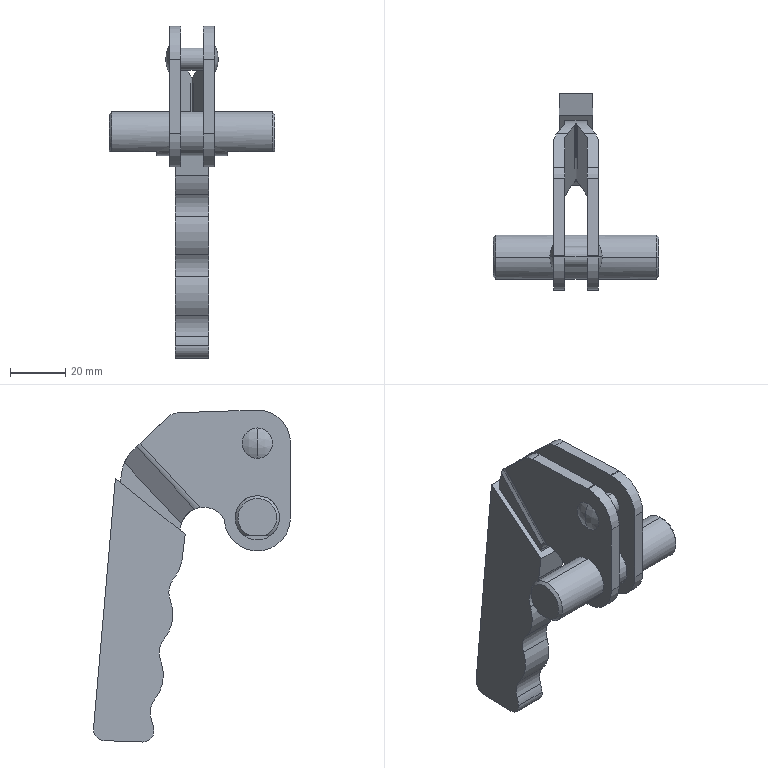Part | STEP file | _2-QC-408710.step | 1 solid | 72 faces | box 60 x 71.267 x 120.088 mm | volume 53013 mm3 | cylinder 35 | plane 30 | sphere 4 | cone 3 | commonest cylinder face diameters 16 x9 8 x8 24 x6 28 x4 17 x3 0.2 x2